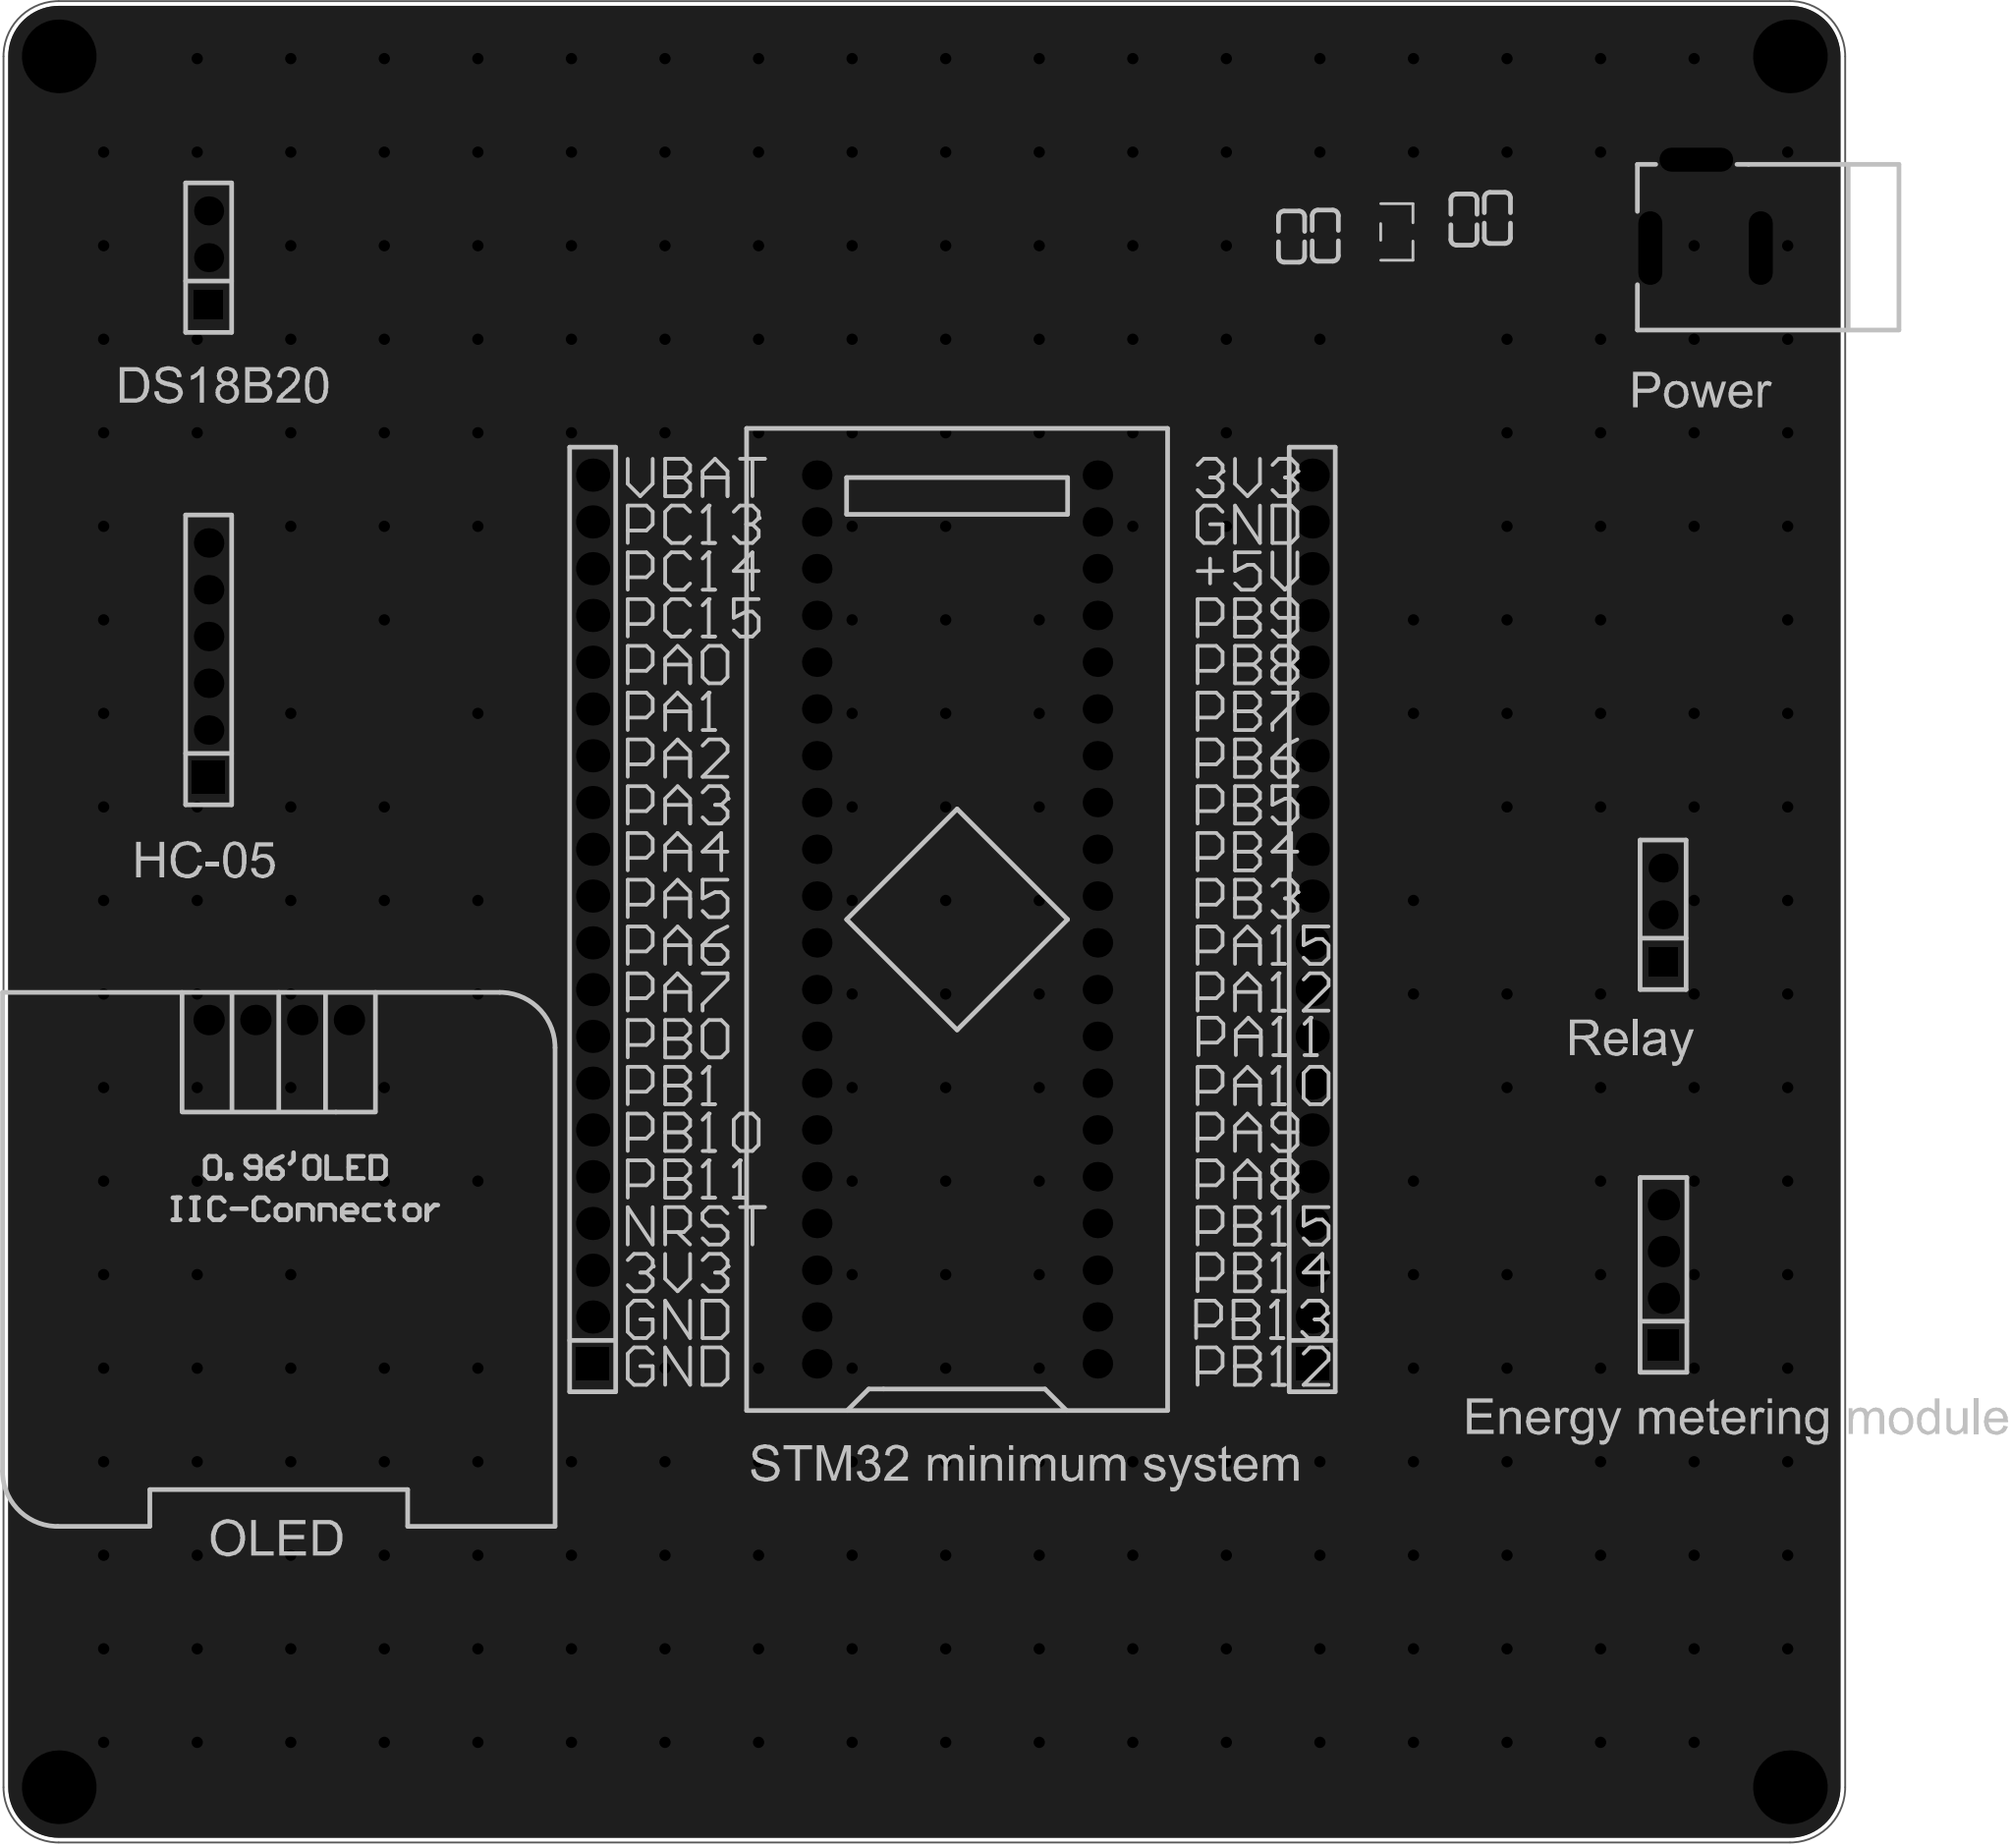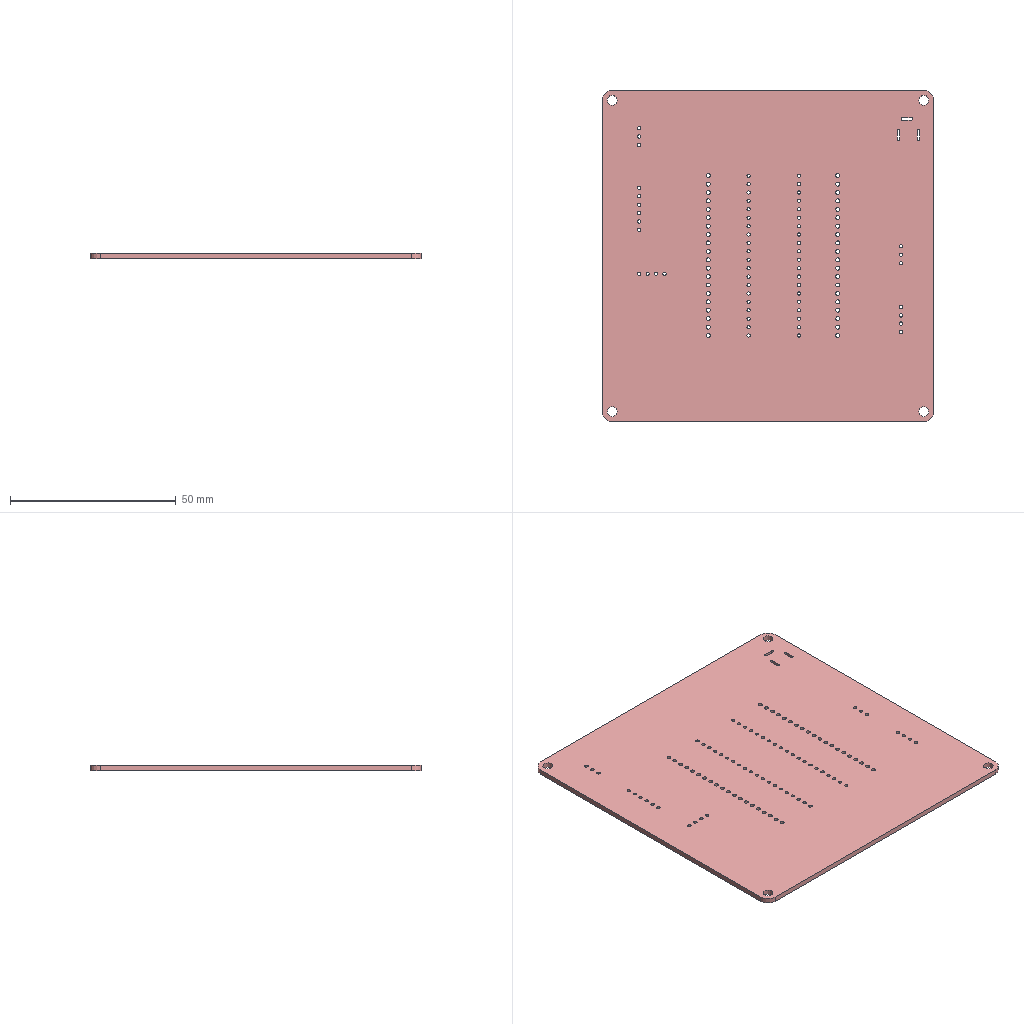Circuit board layout | Altium Designer | box 100 x 100 x 1.6 mm
Layer stack:
# Altium Designer layer stack of  (unit mm; dielectric type: 0 none, 1 core, 2 prepreg, 3 surface material)
index,name,kind,layer,copper_thickness_mm,dielectric_type,dielectric_thickness_mm,dielectric_material,dielectric_constant
0,Top Paste Mask Layer,other,,,,,,
1,Top Silkscreen Layer,other,,,,,,
2,Top Solder Mask Layer,dielectric,,,3,0.01,,3.3
3,Top Layer,copper,Top Layer,0.035,,,,
4,Dielectric1,dielectric,,,3,1.51,FR4,4.5
5,Bottom Layer,copper,Bottom Layer,0.035,,,,
6,Bottom Solder Mask Layer,dielectric,,,3,0.01,,3.3
7,Bottom Silkscreen Layer,other,,,,,,
8,Bottom Paste Mask Layer,other,,,,,,
# drill layer pairs: low layer,high layer
drill_pair,Top Layer,Bottom Layer
Part placement:
Designator,Comment,Layer,Footprint,Center-X(mm),Center-Y(mm),Rotation
U1,STM32F103C8T6-Card,TopLayer,CONN-TH_L53.3-W22.9_STM32F103C8T6-CARD,132.334,129.032,90
H1,,TopLayer,HDR-TH_20P-P2.54-V-F,151.617,129.032,90
H2,,TopLayer,HDR-TH_20P-P2.54-V-F,112.546,129.032,90
C1,10uF,TopLayer,C0603,161.671,167.132,270
C2,100nF,TopLayer,C0603,159.854,167.043,270
C3,10uF,TopLayer,C0603,152.326,166.169,270
C4,100nF,TopLayer,C0603,150.495,166.116,270
DC1,,TopLayer,DC-2.0,172.974,167.894,0
U2,HT7333,TopLayer,SOT-23-3_L2.9-W1.6-P1.90-LS2.8-BR,156.21,166.37,180
H4,,TopLayer,HDR-TH_6P-P2.54-V-F,91.694,143.129,90
H5,,TopLayer,HDR-TH_4P-P2.54-V-F,170.688,109.728,90
H6,,TopLayer,HDR-TH_3P-P2.54-V-F,170.668,129.286,90
OLED1,,TopLayer,0.96OLED_4P,95.504,123.571,0
H3,,TopLayer,HDR-TH_3P-P2.54-V-F,91.694,164.973,90
Pad and via stacks:
# Altium Designer via and pad stacks of  (unit mm). Each distinct definition once, with the count of objects using it.
# via: kind,start_layer,end_layer,hole_mm,diameter_mm,mode(0 simple;1 top-mid-bottom;2 full stack),diameter_per_layer,count,example_net
# pad: kind,layer,hole_mm,hole_type(0 round;1 square;2 slot),plating,top_size,top_shape(1 round;2 rect;3 octagon;9 rounded rect),mid_size,bottom_size,mode,footprint,size_per_layer,count,example
pad,Multi-Layer,3,0,plated,4x4,1,4x4,4x4,0,,,4,1
pad,Multi-Layer,1,0,plated,1.6x1.6,1,1.6x1.6,1.6x1.6,0,CONN-TH_L53.3-W22.9_STM32F103C8T6-CARD,,40,U1.1
pad,Multi-Layer,1.2,0,plated,1.8x1.8,2,1.8x1.8,1.8x1.8,0,HDR-TH_20P-P2.54-V-F,,2,H1.1
pad,Multi-Layer,1.2,0,plated,1.8x1.8,1,1.8x1.8,1.8x1.8,0,HDR-TH_20P-P2.54-V-F,,38,H1.2
pad,Multi-Layer,0.8001,2,plated,4x1.3,1,4x1.3,4x1.3,0,DC-2.0,,3,DC1.2
pad,Multi-Layer,1.02,0,plated,1.6x1.6,1,1.6x1.6,1.6x1.6,0,HDR-TH_6P-P2.54-V-F,,5,H4.6
pad,Multi-Layer,1.02,0,plated,1.8x1.8,2,1.8x1.8,1.8x1.8,0,HDR-TH_6P-P2.54-V-F,,1,H4.1
pad,Multi-Layer,1.1,0,plated,1.7x1.7,2,1.7x1.7,1.7x1.7,0,HDR-TH_4P-P2.54-V-F,,1,H5.1
pad,Multi-Layer,1.1,0,plated,1.7x1.7,1,1.7x1.7,1.7x1.7,0,HDR-TH_4P-P2.54-V-F,,3,H5.2
pad,Multi-Layer,1.02,0,plated,1.575x1.575,1,1.575x1.575,1.575x1.575,0,HDR-TH_3P-P2.54-V-F,,4,H6.3
pad,Multi-Layer,1.02,0,plated,1.575x1.575,2,1.575x1.575,1.575x1.575,0,HDR-TH_3P-P2.54-V-F,,2,H6.1
pad,Multi-Layer,1,0,plated,1.65x1.65,1,1.65x1.65,1.65x1.65,0,0.96OLED_4P,,4,OLED1.4
pad,Top Layer,0,0,plated,0.8x0.9,2,0.8x0.9,0.8x0.9,0,C0603,,8,C1.2
pad,Top Layer,0,0,plated,1.07x0.6,2,1.07x0.6,1.07x0.6,0,SOT-23-3_L2.9-W1.6-P1.90-LS2.8-BR,,3,U2.1
via,Top Layer,Bottom Layer,0.3048,0.61,0,,273,GND
Copper pours:
name,layer,net,type(0 solid;1 hatched;2 none)
Bottom Layer-GND,Bottom Layer,GND,0
Top Layer-GND,Top Layer,GND,0